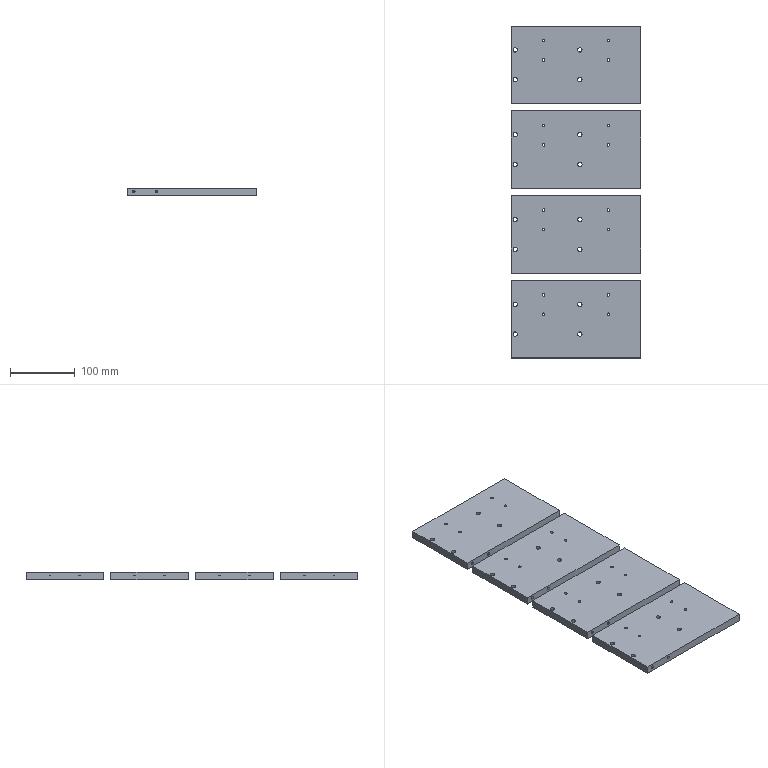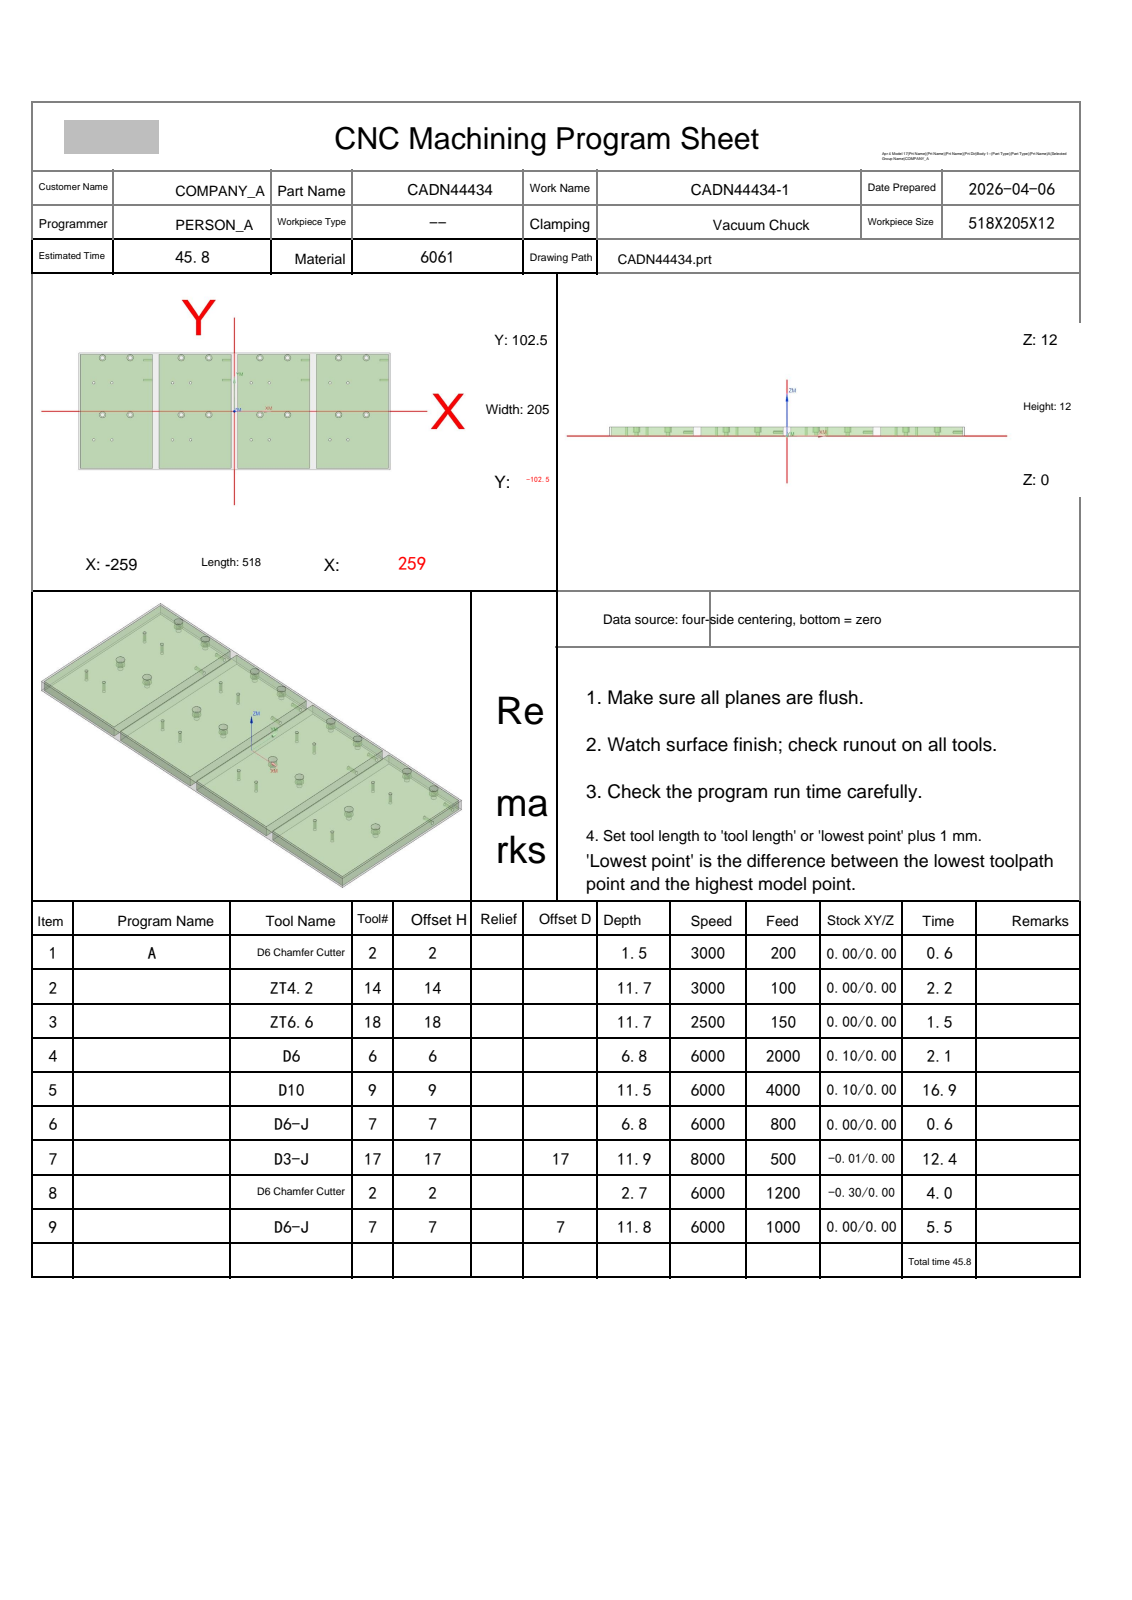NC program | NX | posted by the shop | part box 200 x 513 x 12 mm
Lines 7239 to 7719 of 7719:
N8 T02 M06
(D6 Chamfer Cutter  D=6. R=0. H=02 ce=0.00 di=0.00)
G00 G90 G54 X-134.372 Y.25 M03 S6000
G43 H02 Z32.
M08
Z14.099
G01 Z10.5 F1200.
G03 X-134.672 Y.33 I-.3 J-.52
X-135.192 Y.03 I0.0 J-.6
G01 X-135.2 Y0.0
Y-100.
G02 X-136.5 Y-101.3 I-1.3 J0.0
G01 X-256.5
G02 X-257.8 Y-100. I0.0 J1.3
G01 Y100.
G02 X-256.5 Y101.3 I1.3 J0.0
G01 X-136.5
G02 X-135.2 Y100. I0.0 J-1.3
G01 Y0.0
X-135.192 Y-.03
G03 X-134.672 Y-.33 I.52 J.3
X-134.372 Y-.25 I0.0 J.6
G01 Z14.099
G00 Z14.25
X-127.628
Z14.099
G01 Z10.5
G03 X-127.328 Y-.33 I.3 J.52
X-126.808 Y-.03 I0.0 J.6
G01 X-126.8 Y0.0
Y100.
G02 X-125.5 Y101.3 I1.3 J0.0
G01 X-5.5
G02 X-4.2 Y100. I0.0 J-1.3
G01 Y-100.
G02 X-5.5 Y-101.3 I-1.3 J0.0
G01 X-125.5
G02 X-126.8 Y-100. I0.0 J1.3
G01 Y0.0
X-126.808 Y.03
G03 X-127.328 Y.33 I-.52 J-.3
X-127.628 Y.25 I0.0 J-.6
G01 Z14.099
G00 Z32.
X3.372 Y-.25
Z14.099
G01 Z10.5
G03 X3.672 Y-.33 I.3 J.52
X4.192 Y-.03 I0.0 J.6
G01 X4.2 Y0.0
Y100.
G02 X5.5 Y101.3 I1.3 J0.0
G01 X125.5
G02 X126.8 Y100. I0.0 J-1.3
G01 Y-100.
G02 X125.5 Y-101.3 I-1.3 J0.0
G01 X5.5
G02 X4.2 Y-100. I0.0 J1.3
G01 Y0.0
X4.192 Y.03
G03 X3.672 Y.33 I-.52 J-.3
X3.372 Y.25 I0.0 J-.6
G01 Z14.099
G00 Z32.
X134.372 Y-.25
Z14.099
G01 Z10.5
G03 X134.672 Y-.33 I.3 J.52
X135.192 Y-.03 I0.0 J.6
G01 X135.2 Y0.0
Y100.
G02 X136.5 Y101.3 I1.3 J0.0
G01 X256.5
G02 X257.8 Y100. I0.0 J-1.3
G01 Y-100.
G02 X256.5 Y-101.3 I-1.3 J0.0
G01 X136.5
G02 X135.2 Y-100. I0.0 J1.3
G01 Y0.0
X135.192 Y.03
G03 X134.672 Y.33 I-.52 J-.3
X134.372 Y.25 I0.0 J-.6
G01 Z14.099
G00 Z32.
G00 G90 X-73. Y-50. M03 S5000
Z32.
G98 G81 X-73. Y-50. Z9.333 R15. F150.
X-103.
X-204.
X-234.
Y50.
X-204.
X-103.
X-73.
X28.
X58.
X159.
X189.
Y-50.
X159.
X58.
X28.
G80
G00 Z32.
G00 G90 X-216.795 Y-5.279 M03 S6000
Z32.
Z10.5
G01 Z10. F600.
X-216.5 Y-5.2
G03 X-219.5 Y-2.2 I-3. J0.0
X-223.3 Y-6. I0.0 J-3.8
X-219.5 Y-9.8 I3.8 J0.0
X-215.7 Y-6. I0.0 J3.8
X-219.5 Y-2.2 I-3.8 J0.0
X-222.5 Y-5.2 I0.0 J-3.
G01 X-222.205 Y-5.279
Z10.5
G00 Z32.
X-170.795
Z10.5
G01 Z10.
X-170.5 Y-5.2
G03 X-173.5 Y-2.2 I-3. J0.0
X-177.3 Y-6. I0.0 J-3.8
X-173.5 Y-9.8 I3.8 J0.0
X-169.7 Y-6. I0.0 J3.8
X-173.5 Y-2.2 I-3.8 J0.0
X-176.5 Y-5.2 I0.0 J-3.
G01 X-176.205 Y-5.279
Z10.5
G00 Z32.
X-85.795
Z10.5
G01 Z10.
X-85.5 Y-5.2
G03 X-88.5 Y-2.2 I-3. J0.0
X-92.3 Y-6. I0.0 J-3.8
X-88.5 Y-9.8 I3.8 J0.0
X-84.7 Y-6. I0.0 J3.8
X-88.5 Y-2.2 I-3.8 J0.0
X-91.5 Y-5.2 I0.0 J-3.
G01 X-91.205 Y-5.279
Z10.5
G00 Z32.
X-39.795
Z10.5
G01 Z10.
X-39.5 Y-5.2
G03 X-42.5 Y-2.2 I-3. J0.0
X-46.3 Y-6. I0.0 J-3.8
X-42.5 Y-9.8 I3.8 J0.0
X-38.7 Y-6. I0.0 J3.8
X-42.5 Y-2.2 I-3.8 J0.0
X-45.5 Y-5.2 I0.0 J-3.
G01 X-45.205 Y-5.279
Z10.5
G00 Z32.
X45.205
Z10.5
G01 Z10.
X45.5 Y-5.2
G03 X42.5 Y-2.2 I-3. J0.0
X38.7 Y-6. I0.0 J-3.8
X42.5 Y-9.8 I3.8 J0.0
X46.3 Y-6. I0.0 J3.8
X42.5 Y-2.2 I-3.8 J0.0
X39.5 Y-5.2 I0.0 J-3.
G01 X39.795 Y-5.279
Z10.5
G00 Z32.
X91.205
Z10.5
G01 Z10.
X91.5 Y-5.2
G03 X88.5 Y-2.2 I-3. J0.0
X84.7 Y-6. I0.0 J-3.8
X88.5 Y-9.8 I3.8 J0.0
X92.3 Y-6. I0.0 J3.8
X88.5 Y-2.2 I-3.8 J0.0
X85.5 Y-5.2 I0.0 J-3.
G01 X85.795 Y-5.279
Z10.5
G00 Z32.
X176.205
Z10.5
G01 Z10.
X176.5 Y-5.2
G03 X173.5 Y-2.2 I-3. J0.0
X169.7 Y-6. I0.0 J-3.8
X173.5 Y-9.8 I3.8 J0.0
X177.3 Y-6. I0.0 J3.8
X173.5 Y-2.2 I-3.8 J0.0
X170.5 Y-5.2 I0.0 J-3.
G01 X170.795 Y-5.279
Z10.5
G00 Z32.
X222.205
Z10.5
G01 Z10.
X222.5 Y-5.2
G03 X219.5 Y-2.2 I-3. J0.0
X215.7 Y-6. I0.0 J-3.8
X219.5 Y-9.8 I3.8 J0.0
X223.3 Y-6. I0.0 J3.8
X219.5 Y-2.2 I-3.8 J0.0
X216.5 Y-5.2 I0.0 J-3.
G01 X216.795 Y-5.279
Z10.5
G00 Z32.
X222.205 Y94.721
Z10.5
G01 Z10.
X222.5 Y94.8
G03 X219.5 Y97.8 I-3. J0.0
X215.7 Y94. I0.0 J-3.8
X219.5 Y90.2 I3.8 J0.0
X223.3 Y94. I0.0 J3.8
X219.5 Y97.8 I-3.8 J0.0
X216.5 Y94.8 I0.0 J-3.
G01 X216.795 Y94.721
Z10.5
G00 Z32.
X176.205
Z10.5
G01 Z10.
X176.5 Y94.8
G03 X173.5 Y97.8 I-3. J0.0
X169.7 Y94. I0.0 J-3.8
X173.5 Y90.2 I3.8 J0.0
X177.3 Y94. I0.0 J3.8
X173.5 Y97.8 I-3.8 J0.0
X170.5 Y94.8 I0.0 J-3.
G01 X170.795 Y94.721
Z10.5
G00 Z32.
X91.205
Z10.5
G01 Z10.
X91.5 Y94.8
G03 X88.5 Y97.8 I-3. J0.0
X84.7 Y94. I0.0 J-3.8
X88.5 Y90.2 I3.8 J0.0
X92.3 Y94. I0.0 J3.8
X88.5 Y97.8 I-3.8 J0.0
X85.5 Y94.8 I0.0 J-3.
G01 X85.795 Y94.721
Z10.5
G00 Z32.
X45.205
Z10.5
G01 Z10.
X45.5 Y94.8
G03 X42.5 Y97.8 I-3. J0.0
X38.7 Y94. I0.0 J-3.8
X42.5 Y90.2 I3.8 J0.0
X46.3 Y94. I0.0 J3.8
X42.5 Y97.8 I-3.8 J0.0
X39.5 Y94.8 I0.0 J-3.
G01 X39.795 Y94.721
Z10.5
G00 Z32.
X-39.795
Z10.5
G01 Z10.
X-39.5 Y94.8
G03 X-42.5 Y97.8 I-3. J0.0
X-46.3 Y94. I0.0 J-3.8
X-42.5 Y90.2 I3.8 J0.0
X-38.7 Y94. I0.0 J3.8
X-42.5 Y97.8 I-3.8 J0.0
X-45.5 Y94.8 I0.0 J-3.
G01 X-45.205 Y94.721
Z10.5
G00 Z32.
X-85.795
Z10.5
G01 Z10.
X-85.5 Y94.8
G03 X-88.5 Y97.8 I-3. J0.0
X-92.3 Y94. I0.0 J-3.8
X-88.5 Y90.2 I3.8 J0.0
X-84.7 Y94. I0.0 J3.8
X-88.5 Y97.8 I-3.8 J0.0
X-91.5 Y94.8 I0.0 J-3.
G01 X-91.205 Y94.721
Z10.5
G00 Z32.
X-170.795
Z10.5
G01 Z10.
X-170.5 Y94.8
G03 X-173.5 Y97.8 I-3. J0.0
X-177.3 Y94. I0.0 J-3.8
X-173.5 Y90.2 I3.8 J0.0
X-169.7 Y94. I0.0 J3.8
X-173.5 Y97.8 I-3.8 J0.0
X-176.5 Y94.8 I0.0 J-3.
G01 X-176.205 Y94.721
Z10.5
G00 Z32.
X-216.795
Z10.5
G01 Z10.
X-216.5 Y94.8
G03 X-219.5 Y97.8 I-3. J0.0
X-223.3 Y94. I0.0 J-3.8
X-219.5 Y90.2 I3.8 J0.0
X-215.7 Y94. I0.0 J3.8
X-219.5 Y97.8 I-3.8 J0.0
X-222.5 Y94.8 I0.0 J-3.
G01 X-222.205 Y94.721
Z10.5
G00 Z32.
G91 G28 Z0.0
M05
M09
G91 G28 Z0.0
M01
N9 T07 M06
(D6-J  D=6. R=0. H=07 ce=0.00 di=0.00)
G00 G90 G54 X-260.573 Y-101.017 M03 S6000
G43 H07 Z32.
M08
Z1.
G01 Z.5 F1000.
G41 D07
X-260.375 Y-100.992
G03 X-259.5 Y-100. I-.125 J.992
G01 Y100.
G02 X-256.5 Y103. I3. J0.0
G01 X-136.5
G02 X-133.5 Y100. I0.0 J-3.
G01 Y-100.
G02 X-136.5 Y-103. I-3. J0.0
G01 X-256.5
G02 X-259.5 Y-100. I0.0 J3.
G01 Y-99.5
G03 X-260.5 Y-98.5 I-1. J0.0
G01 G40 X-260.7
Z1.
G00 Z32.
X-129.573 Y-101.017
Z1.
G01 Z.5
G41 D07
X-129.375 Y-100.992
G03 X-128.5 Y-100. I-.125 J.992
G01 Y100.
G02 X-125.5 Y103. I3. J0.0
G01 X-5.5
G02 X-2.5 Y100. I0.0 J-3.
G01 Y-100.
G02 X-5.5 Y-103. I-3. J0.0
G01 X-125.5
G02 X-128.5 Y-100. I0.0 J3.
G01 Y-99.5
G03 X-129.5 Y-98.5 I-1. J0.0
G01 G40 X-129.7
Z1.
G00 Z32.
X1.427 Y-101.017
Z1.
G01 Z.5
G41 D07
X1.625 Y-100.992
G03 X2.5 Y-100. I-.125 J.992
G01 Y100.
G02 X5.5 Y103. I3. J0.0
G01 X125.5
G02 X128.5 Y100. I0.0 J-3.
G01 Y-100.
G02 X125.5 Y-103. I-3. J0.0
G01 X5.5
G02 X2.5 Y-100. I0.0 J3.
G01 Y-99.5
G03 X1.5 Y-98.5 I-1. J0.0
G01 G40 X1.3
Z1.
G00 Z32.
X260.573 Y101.017
Z1.
G01 Z.5
G41 D07
X260.375 Y100.992
G03 X259.5 Y100. I.125 J-.992
G01 Y-100.
G02 X256.5 Y-103. I-3. J0.0
G01 X136.5
G02 X133.5 Y-100. I0.0 J3.
G01 Y100.
G02 X136.5 Y103. I3. J0.0
G01 X256.5
G02 X259.5 Y100. I0.0 J-3.
G01 Y99.5
G03 X260.5 Y98.5 I1. J0.0
G01 G40 X260.7
Z1.
G00 Z32.
G00 G90 X-260.474 Y-101.005 M03 S6000
Z32.
Z.7
G01 Z.2 F1000.
G41 D07
X-260.375 Y-100.992
G03 X-259.5 Y-100. I-.125 J.992
G01 Y100.
G02 X-256.5 Y103. I3. J0.0
G01 X-136.5
G02 X-133.5 Y100. I0.0 J-3.
G01 Y-100.
G02 X-136.5 Y-103. I-3. J0.0
G01 X-256.5
G02 X-259.5 Y-100. I0.0 J3.
G01 Y-99.5
G03 X-260.5 Y-98.5 I-1. J0.0
G01 G40 X-260.6
Z.7
G00 Z32.
X-129.474 Y-101.005
Z.7
G01 Z.2
G41 D07
X-129.375 Y-100.992
G03 X-128.5 Y-100. I-.125 J.992
G01 Y100.
G02 X-125.5 Y103. I3. J0.0
G01 X-5.5
G02 X-2.5 Y100. I0.0 J-3.
G01 Y-100.
G02 X-5.5 Y-103. I-3. J0.0
G01 X-125.5
G02 X-128.5 Y-100. I0.0 J3.
G01 Y-99.5
G03 X-129.5 Y-98.5 I-1. J0.0
G01 G40 X-129.6
Z.7
G00 Z32.
X1.526 Y-101.005
Z.7
G01 Z.2
G41 D07
X1.625 Y-100.992
G03 X2.5 Y-100. I-.125 J.992
G01 Y100.
G02 X5.5 Y103. I3. J0.0
G01 X125.5
G02 X128.5 Y100. I0.0 J-3.
G01 Y-100.
G02 X125.5 Y-103. I-3. J0.0
G01 X5.5
G02 X2.5 Y-100. I0.0 J3.
G01 Y-99.5
G03 X1.5 Y-98.5 I-1. J0.0
G01 G40 X1.4
Z.7
G00 Z32.
X260.474 Y101.005
Z.7
G01 Z.2
G41 D07
X260.375 Y100.992
G03 X259.5 Y100. I.125 J-.992
G01 Y-100.
G02 X256.5 Y-103. I-3. J0.0
G01 X136.5
G02 X133.5 Y-100. I0.0 J3.
G01 Y100.
G02 X136.5 Y103. I3. J0.0
G01 X256.5
G02 X259.5 Y100. I0.0 J-3.
G01 Y99.5
G03 X260.5 Y98.5 I1. J0.0
G01 G40 X260.6
Z.7
G00 Z32.
M05
M09
G91 G28 Z0.0
G91 G28 Y0.0
M30
%